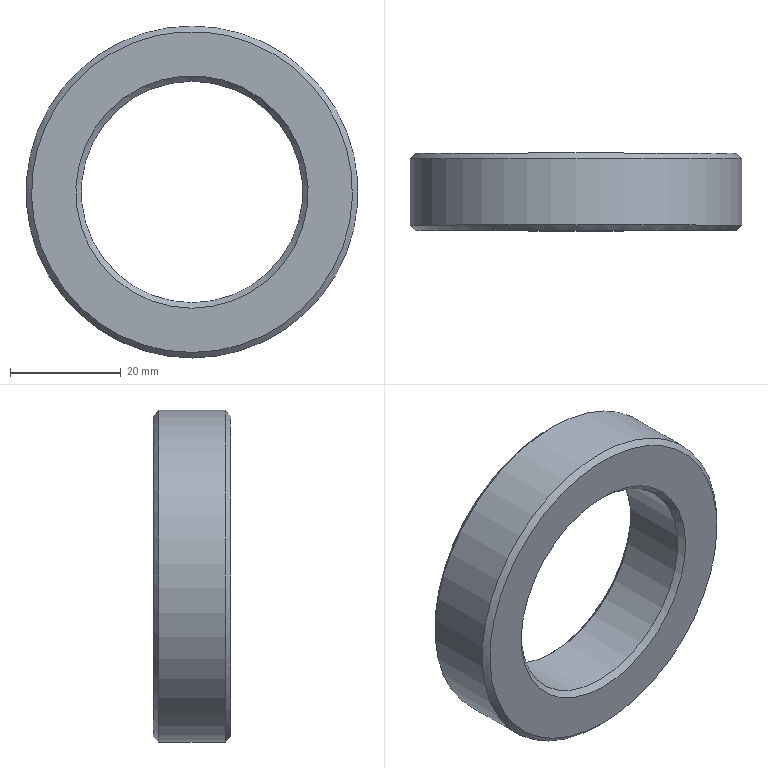Part | NX | features BREP 1, DATUM_CSYS 1 | 1 solid | 8 faces | box 60 x 14 x 60 mm | volume 21677 mm3 | cone 4 | cylinder 2 | plane 2 | commonest cylinder face diameters 40 x1 60 x1
STEP:
#1=CARTESIAN_POINT('',(0.,589.,-30.));
#2=VERTEX_POINT('',#1);
#3=CARTESIAN_POINT('',(0.,589.,0.));
#4=DIRECTION('',(0.,-1.,0.));
#5=DIRECTION('',(0.,0.,-1.));
#6=AXIS2_PLACEMENT_3D('',#3,#4,#5);
#7=CIRCLE('',#6,30.);
#8=EDGE_CURVE('',#2,#2,#7,.T.);
#9=ORIENTED_EDGE('',*,*,#8,.F.);
#10=EDGE_LOOP('',(#9));
#11=FACE_BOUND('',#10,.T.);
#12=CARTESIAN_POINT('',(0.,601.,-30.));
#13=VERTEX_POINT('',#12);
#14=CARTESIAN_POINT('',(0.,601.,0.));
#15=DIRECTION('',(0.,-1.,0.));
#16=DIRECTION('',(0.,0.,-1.));
#17=AXIS2_PLACEMENT_3D('',#14,#15,#16);
#18=CIRCLE('',#17,30.);
#19=EDGE_CURVE('',#13,#13,#18,.T.);
#20=ORIENTED_EDGE('',*,*,#19,.T.);
#21=EDGE_LOOP('',(#20));
#22=FACE_BOUND('',#21,.T.);
#23=CARTESIAN_POINT('',(0.,604.,0.));
#24=DIRECTION('',(0.,-1.,0.));
#25=DIRECTION('',(0.,0.,-1.));
#26=AXIS2_PLACEMENT_3D('',#23,#24,#25);
#27=CYLINDRICAL_SURFACE('',#26,30.);
#28=ADVANCED_FACE('',(#11,#22),#27,.T.);
#29=CARTESIAN_POINT('',(0.,588.,-29.));
#30=VERTEX_POINT('',#29);
#31=CARTESIAN_POINT('',(0.,588.,0.));
#32=DIRECTION('',(0.,-1.,0.));
#33=DIRECTION('',(0.,0.,-1.));
#34=AXIS2_PLACEMENT_3D('',#31,#32,#33);
#35=CIRCLE('',#34,29.);
#36=EDGE_CURVE('',#30,#30,#35,.T.);
#37=ORIENTED_EDGE('',*,*,#36,.F.);
#38=EDGE_LOOP('',(#37));
#39=FACE_BOUND('',#38,.T.);
#40=ORIENTED_EDGE('',*,*,#8,.T.);
#41=EDGE_LOOP('',(#40));
#42=FACE_BOUND('',#41,.T.);
#43=CARTESIAN_POINT('',(0.,589.,0.));
#44=DIRECTION('',(0.,1.,0.));
#45=DIRECTION('',(0.,0.,1.));
#46=AXIS2_PLACEMENT_3D('',#43,#44,#45);
#47=CONICAL_SURFACE('',#46,30.,0.7854);
#48=ADVANCED_FACE('',(#39,#42),#47,.T.);
#49=CARTESIAN_POINT('',(0.,588.,-21.));
#50=VERTEX_POINT('',#49);
#51=CARTESIAN_POINT('',(0.,588.,0.));
#52=DIRECTION('',(0.,-1.,0.));
#53=DIRECTION('',(0.,0.,-1.));
#54=AXIS2_PLACEMENT_3D('',#51,#52,#53);
#55=CIRCLE('',#54,21.);
#56=EDGE_CURVE('',#50,#50,#55,.T.);
#57=ORIENTED_EDGE('',*,*,#56,.F.);
#58=EDGE_LOOP('',(#57));
#59=FACE_BOUND('',#58,.T.);
#60=ORIENTED_EDGE('',*,*,#36,.T.);
#61=EDGE_LOOP('',(#60));
#62=FACE_BOUND('',#61,.T.);
#63=CARTESIAN_POINT('',(-29.,588.,0.));
#64=DIRECTION('',(0.,1.,0.));
#65=DIRECTION('',(0.,0.,1.));
#66=AXIS2_PLACEMENT_3D('',#63,#64,#65);
#67=PLANE('',#66);
#68=ADVANCED_FACE('',(#59,#62),#67,.F.);
#69=CARTESIAN_POINT('',(0.,589.,-20.));
#70=VERTEX_POINT('',#69);
#71=CARTESIAN_POINT('',(0.,589.,0.));
#72=DIRECTION('',(0.,-1.,0.));
#73=DIRECTION('',(0.,0.,-1.));
#74=AXIS2_PLACEMENT_3D('',#71,#72,#73);
#75=CIRCLE('',#74,20.);
#76=EDGE_CURVE('',#70,#70,#75,.T.);
#77=ORIENTED_EDGE('',*,*,#76,.F.);
#78=EDGE_LOOP('',(#77));
#79=FACE_BOUND('',#78,.T.);
#80=ORIENTED_EDGE('',*,*,#56,.T.);
#81=EDGE_LOOP('',(#80));
#82=FACE_BOUND('',#81,.T.);
#83=CARTESIAN_POINT('',(0.,588.,0.));
#84=DIRECTION('',(0.,-1.,0.));
#85=DIRECTION('',(0.,0.,-1.));
#86=AXIS2_PLACEMENT_3D('',#83,#84,#85);
#87=CONICAL_SURFACE('',#86,21.,0.7854);
#88=ADVANCED_FACE('',(#79,#82),#87,.F.);
#89=CARTESIAN_POINT('',(0.,601.,-20.));
#90=VERTEX_POINT('',#89);
#91=CARTESIAN_POINT('',(0.,601.,0.));
#92=DIRECTION('',(0.,-1.,0.));
#93=DIRECTION('',(0.,0.,-1.));
#94=AXIS2_PLACEMENT_3D('',#91,#92,#93);
#95=CIRCLE('',#94,20.);
#96=EDGE_CURVE('',#90,#90,#95,.T.);
#97=ORIENTED_EDGE('',*,*,#96,.F.);
#98=EDGE_LOOP('',(#97));
#99=FACE_BOUND('',#98,.T.);
#100=ORIENTED_EDGE('',*,*,#76,.T.);
#101=EDGE_LOOP('',(#100));
#102=FACE_BOUND('',#101,.T.);
#103=CARTESIAN_POINT('',(0.,604.,0.));
#104=DIRECTION('',(0.,-1.,0.));
#105=DIRECTION('',(0.,0.,-1.));
#106=AXIS2_PLACEMENT_3D('',#103,#104,#105);
#107=CYLINDRICAL_SURFACE('',#106,20.);
#108=ADVANCED_FACE('',(#99,#102),#107,.F.);
#109=CARTESIAN_POINT('',(0.,602.,-21.));
#110=VERTEX_POINT('',#109);
#111=CARTESIAN_POINT('',(0.,602.,0.));
#112=DIRECTION('',(0.,-1.,0.));
#113=DIRECTION('',(0.,0.,-1.));
#114=AXIS2_PLACEMENT_3D('',#111,#112,#113);
#115=CIRCLE('',#114,21.);
#116=EDGE_CURVE('',#110,#110,#115,.T.);
#117=ORIENTED_EDGE('',*,*,#116,.F.);
#118=EDGE_LOOP('',(#117));
#119=FACE_BOUND('',#118,.T.);
#120=ORIENTED_EDGE('',*,*,#96,.T.);
#121=EDGE_LOOP('',(#120));
#122=FACE_BOUND('',#121,.T.);
#123=CARTESIAN_POINT('',(0.,601.,0.));
#124=DIRECTION('',(0.,1.,0.));
#125=DIRECTION('',(0.,0.,1.));
#126=AXIS2_PLACEMENT_3D('',#123,#124,#125);
#127=CONICAL_SURFACE('',#126,20.,0.7854);
#128=ADVANCED_FACE('',(#119,#122),#127,.F.);
#129=CARTESIAN_POINT('',(0.,602.,-29.));
#130=VERTEX_POINT('',#129);
#131=CARTESIAN_POINT('',(0.,602.,0.));
#132=DIRECTION('',(0.,-1.,0.));
#133=DIRECTION('',(0.,0.,-1.));
#134=AXIS2_PLACEMENT_3D('',#131,#132,#133);
#135=CIRCLE('',#134,29.);
#136=EDGE_CURVE('',#130,#130,#135,.T.);
#137=ORIENTED_EDGE('',*,*,#136,.F.);
#138=EDGE_LOOP('',(#137));
#139=FACE_BOUND('',#138,.T.);
#140=ORIENTED_EDGE('',*,*,#116,.T.);
#141=EDGE_LOOP('',(#140));
#142=FACE_BOUND('',#141,.T.);
#143=CARTESIAN_POINT('',(-21.,602.,0.));
#144=DIRECTION('',(0.,-1.,0.));
#145=DIRECTION('',(0.,0.,-1.));
#146=AXIS2_PLACEMENT_3D('',#143,#144,#145);
#147=PLANE('',#146);
#148=ADVANCED_FACE('',(#139,#142),#147,.F.);
#149=ORIENTED_EDGE('',*,*,#19,.F.);
#150=EDGE_LOOP('',(#149));
#151=FACE_BOUND('',#150,.T.);
#152=ORIENTED_EDGE('',*,*,#136,.T.);
#153=EDGE_LOOP('',(#152));
#154=FACE_BOUND('',#153,.T.);
#155=CARTESIAN_POINT('',(0.,602.,0.));
#156=DIRECTION('',(0.,-1.,0.));
#157=DIRECTION('',(0.,0.,-1.));
#158=AXIS2_PLACEMENT_3D('',#155,#156,#157);
#159=CONICAL_SURFACE('',#158,29.,0.7854);
#160=ADVANCED_FACE('',(#151,#154),#159,.T.);
#161=CLOSED_SHELL('',(#28,#48,#68,#88,#108,#128,#148,#160));
#162=MANIFOLD_SOLID_BREP('',#161);
#163=(LENGTH_UNIT()NAMED_UNIT(*)SI_UNIT(.MILLI.,.METRE.));
#164=UNCERTAINTY_MEASURE_WITH_UNIT(LENGTH_MEASURE(0.00001),#163,'','');
#165=(NAMED_UNIT(*)PLANE_ANGLE_UNIT()SI_UNIT($,.RADIAN.));
#166=(NAMED_UNIT(*)SI_UNIT($,.STERADIAN.)SOLID_ANGLE_UNIT());
#167=(GEOMETRIC_REPRESENTATION_CONTEXT(3)GLOBAL_UNCERTAINTY_ASSIGNED_CONTEXT((#164))GLOBAL_UNIT_ASSIGNED_CONTEXT((#163,#165,#166))REPRESENTATION_CONTEXT('',''));
#168=ADVANCED_BREP_SHAPE_REPRESENTATION('',(#162),#167);